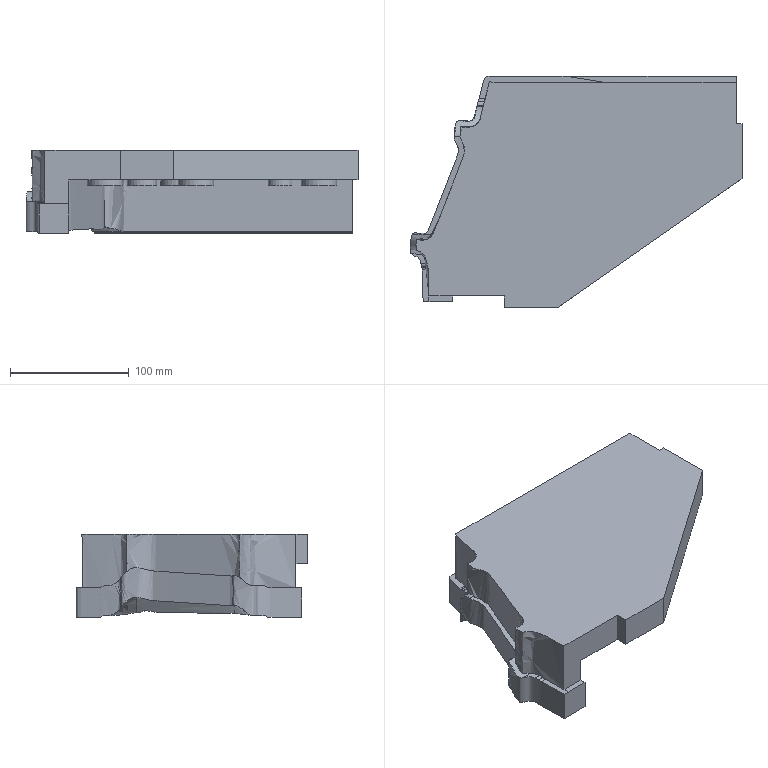Part | NX | features solid 2 | 1 solid | 56 faces | box 279.555 x 195.049 x 70.236 mm | volume 1412452 mm3 | spline 33 | plane 17 | cylinder 6 | commonest cylinder face diameters 30 x4 20 x1 25 x1